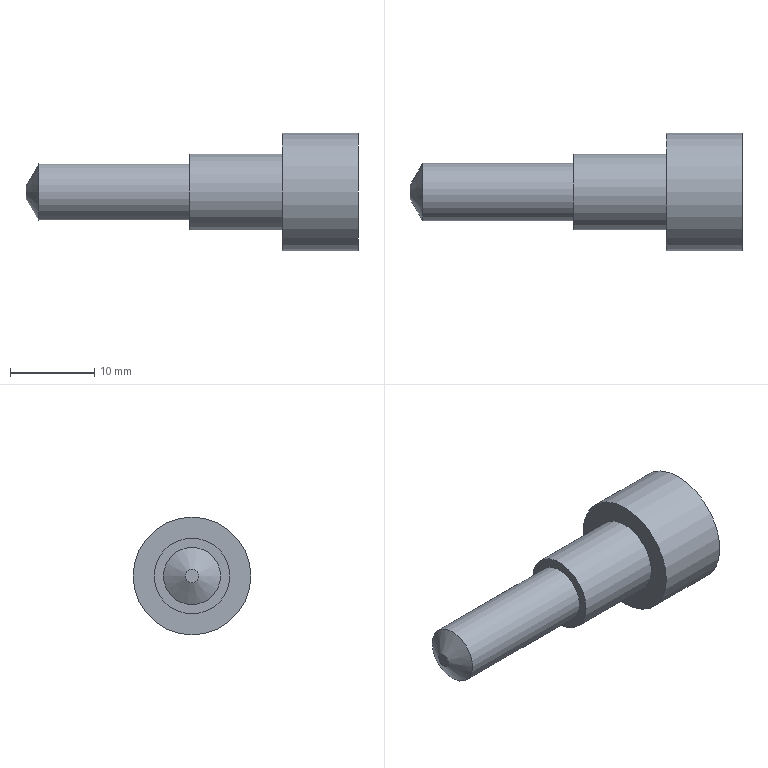Part | STEP file | solid 211 | 1 solid | 8 faces | box 39.5 x 14 x 14 mm | volume 2762 mm3 | plane 4 | cylinder 3 | cone 1 | commonest cylinder face diameters 6.8 x1 9 x1 14 x1